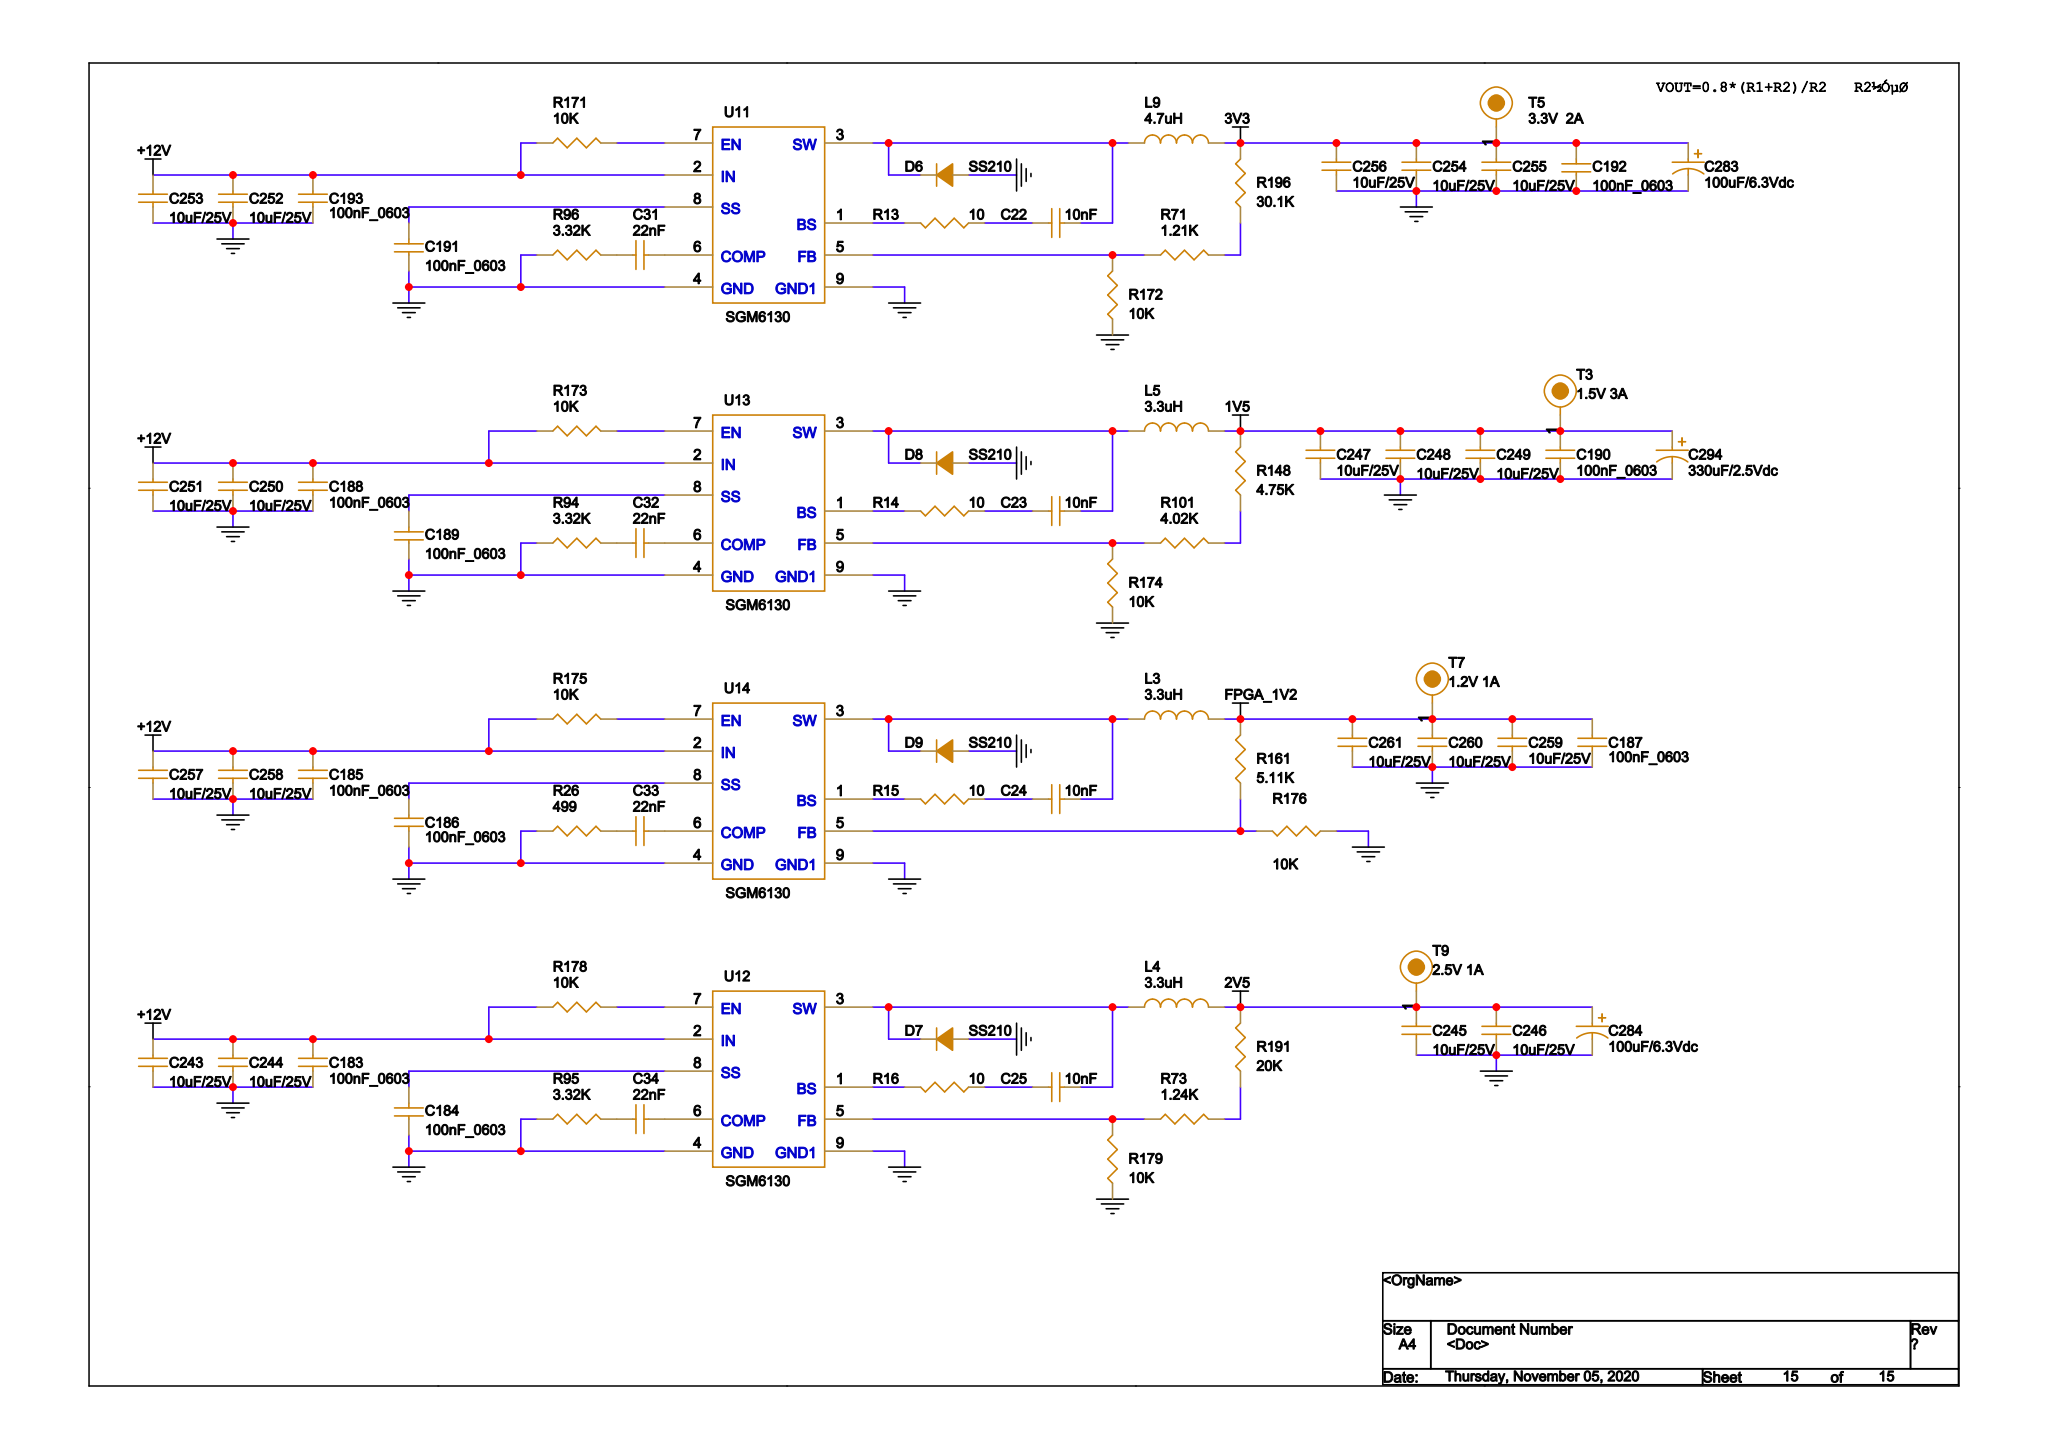Circuit board | Cadence Allegro | 406 parts | 392 nets | one sheet of the schematic
Parts on this sheet (reference | value | footprint):
C22 | 10nF | C_0603
C23 | 10nF | C_0603
C24 | 10nF | C_0603
C25 | 10nF | C_0603
C31 | 22nF | C_0603
C32 | 22nF | C_0603
C33 | 22nF | C_0603
C34 | 22nF | C_0603
C183 | 100nF_0603 | C_0603_104
C184 | 100nF_0603 | C_0603_104
C185 | 100nF_0603 | C_0603_104
C186 | 100nF_0603 | C_0603_104
C187 | 100nF_0603 | C_0603_104
C188 | 100nF_0603 | C_0603_104
C189 | 100nF_0603 | C_0603_104
C190 | 100nF_0603 | C_0603_104
C191 | 100nF_0603 | C_0603_104
C192 | 100nF_0603 | C_0603_104
C193 | 100nF_0603 | C_0603_104
C243 | 10uF/25V | C_0805_106
C244 | 10uF/25V | C_0805_106
C245 | 10uF/25V | C_0805_106
C246 | 10uF/25V | C_0805_106
C247 | 10uF/25V | C_0805_106
C248 | 10uF/25V | C_0805_106
C249 | 10uF/25V | C_0805_106
C250 | 10uF/25V | C_0805_106
C251 | 10uF/25V | C_0805_106
C252 | 10uF/25V | C_0805_106
C253 | 10uF/25V | C_0805_106
C254 | 10uF/25V | C_0805_106
C255 | 10uF/25V | C_0805_106
C256 | 10uF/25V | C_0805_106
C257 | 10uF/25V | C_0805_106
C258 | 10uF/25V | C_0805_106
C259 | 10uF/25V | C_0805_106
C260 | 10uF/25V | C_0805_106
C261 | 10uF/25V | C_0805_106
C283 | 100uF/6.3Vdc | C_7343
C284 | 100uF/6.3Vdc | C_7343
C294 | 330uF/2.5Vdc | C_7343
D6 | SS210 | DO214
D7 | SS210 | DO214
D8 | SS210 | DO214
D9 | SS210 | DO214
L3 | 3.3uH | L_SDB0530
L4 | 3.3uH | L_SDB0530
L5 | 3.3uH | L_SDB0530
L9 | 4.7uH | L_SDB0530
R14 | 10 | R_0603
R15 | 10 | R_0603
R16 | 10 | R_0603
R26 | 499 | R_0603
R71 | 1.21K | R_0603
R73 | 1.24K | R_0603
R94 | 3.32K | R_0603
R95 | 3.32K | R_0603
R96 | 3.32K | R_0603
R101 | 4.02K | R_0603
R148 | 4.75K | R_0603
R161 | 5.11K | R_0603
R171 | 10K | R_0603
R172 | 10K | R_0603
R173 | 10K | R_0603
R174 | 10K | R_0603
R175 | 10K | R_0603
R176 | 10K | R_0603
R178 | 10K | R_0603
R179 | 10K | R_0603
R191 | 20K | R_0603
R196 | 30.1K | R_0603
T3 | 1.5V 3A | TP
T5 | 3.3V  2A | TP
T7 | 1.2V 1A | TP
U11 | SGM6130 | U_SO8DDA
U12 | SGM6130 | U_SO8DDA
U13 | SGM6130 | U_SO8DDA
U14 | SGM6130 | U_SO8DDA
Nets of these parts (net: part-pin ...):
GND: C183-2 C184-1 C185-2 C186-2 C187-2 C188-2 C189-1 C190-2 C191-1 C192-1 C193-2 C243-2 C244-2 C245-2 C246-2 C247-2 C248-2 C249-2 C250-2 C251-2 C252-2 C253-2 C254-2 C255-2 C256-2 C257-2 C258-2 C259-2 C260-2 C261-2 C283-2 C284-2 C294-2 D6-1 D7-1 D8-1 D9-1 R26-1 R94-1 R95-1 R96-1 R172-1 R174-1 R176-1 R179-1 U11-4 U11-9 U12-4 U12-9 U13-4 U13-9 U14-4 U14-9
+12V: C183-1 C185-1 C188-1 C193-1 C243-1 C244-1 C250-1 C251-1 C252-1 C253-1 C257-1 C258-1 R171-1 R173-1 R175-1 R178-1 U11-2 U12-2 U13-2 U14-2
FPGA_1V2: C187-1 C259-1 C260-1 C261-1 L3-2 R161-2 T7-1
3V3: C192-2 C254-1 C255-1 C256-1 C283-1 L9-2 R196-2 T5-1
N20036050: C184-2 U12-8
N20035071: C186-1 U14-8
N20035270: C189-2 U13-8
1V5: C190-1 C247-1 C248-1 C249-1 C294-1 L5-2 R148-2 T3-1
N20035662: C191-2 U11-8
N20035680: C22-1
N20035543: C22-2 D6-2 L9-1 U11-3
N20035290: C23-1 R14-1
N20035002: C23-2 D8-2 L5-1 U13-3
N20035081: C24-1 R15-1
N20035026: C24-2 D9-2 L3-1 U14-3
N20036078: C25-1 R16-1
N20036020: C25-2 D7-2 L4-1 U12-3
2V5: C245-1 C246-1 C284-1 L4-2 R191-2
N200356261: C31-1 R96-2
N200355785: C31-2 U11-6
N200352521: C32-1 R94-2
N200350455: C32-2 U13-6
N200351430: C33-1 R26-2
N200351431: C33-2 U14-6
N200349681: C34-1 R95-2
N200361201: C34-2 U12-6
N20035095: R101-1 R174-2 U13-5
N20035097: R101-2 R148-1
N20035678: U11-1
N20035288: R14-2 U13-1
N20035083: R15-2 U14-1
N20036076: R16-2 U12-1
N20034807: R161-1 R176-2 U14-5
N20035551: R171-2 U11-7
N20035582: R71-1 R172-2 U11-5
N20035010: R173-2 U13-7
N20035053: R175-2 U14-7
N20036036: R178-2 U12-7
N20034929: R73-1 R179-2 U12-5
N20034939: R73-2 R191-1
N20035584: R71-2 R196-1